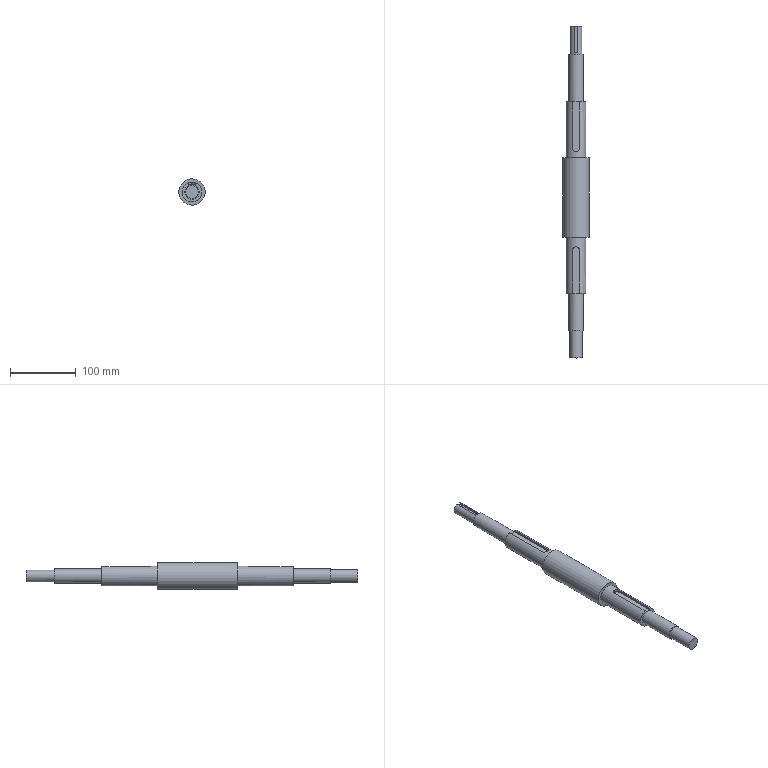Part | STEP file | SN10_001_008_EIXO | 1 solid | 33 faces | box 40 x 503.3 x 40 mm | volume 336623 mm3 | plane 20 | cylinder 13 | commonest cylinder face diameters 8 x4 5 x2 22 x2 30 x2 18 x1 19.05 x1